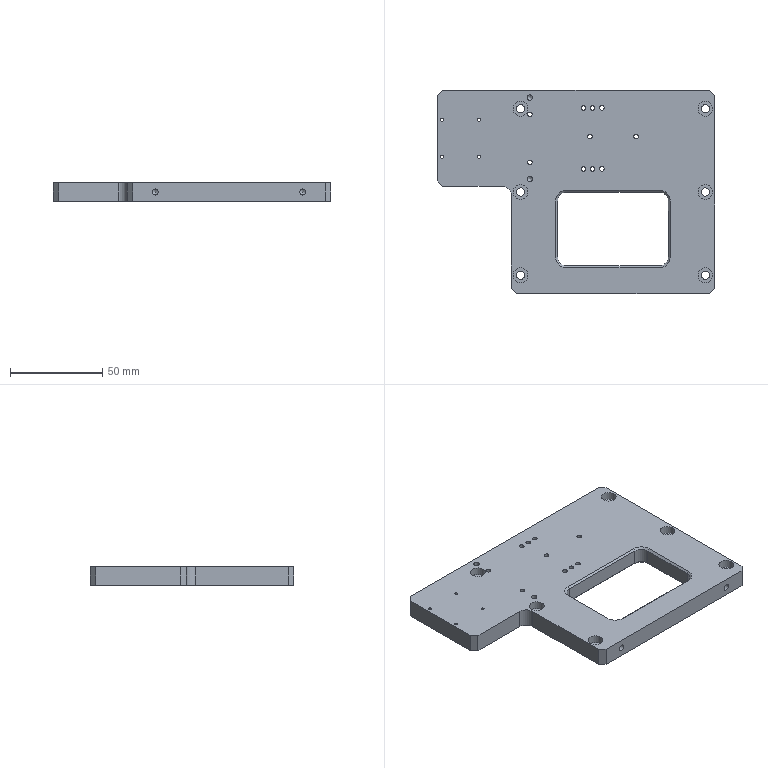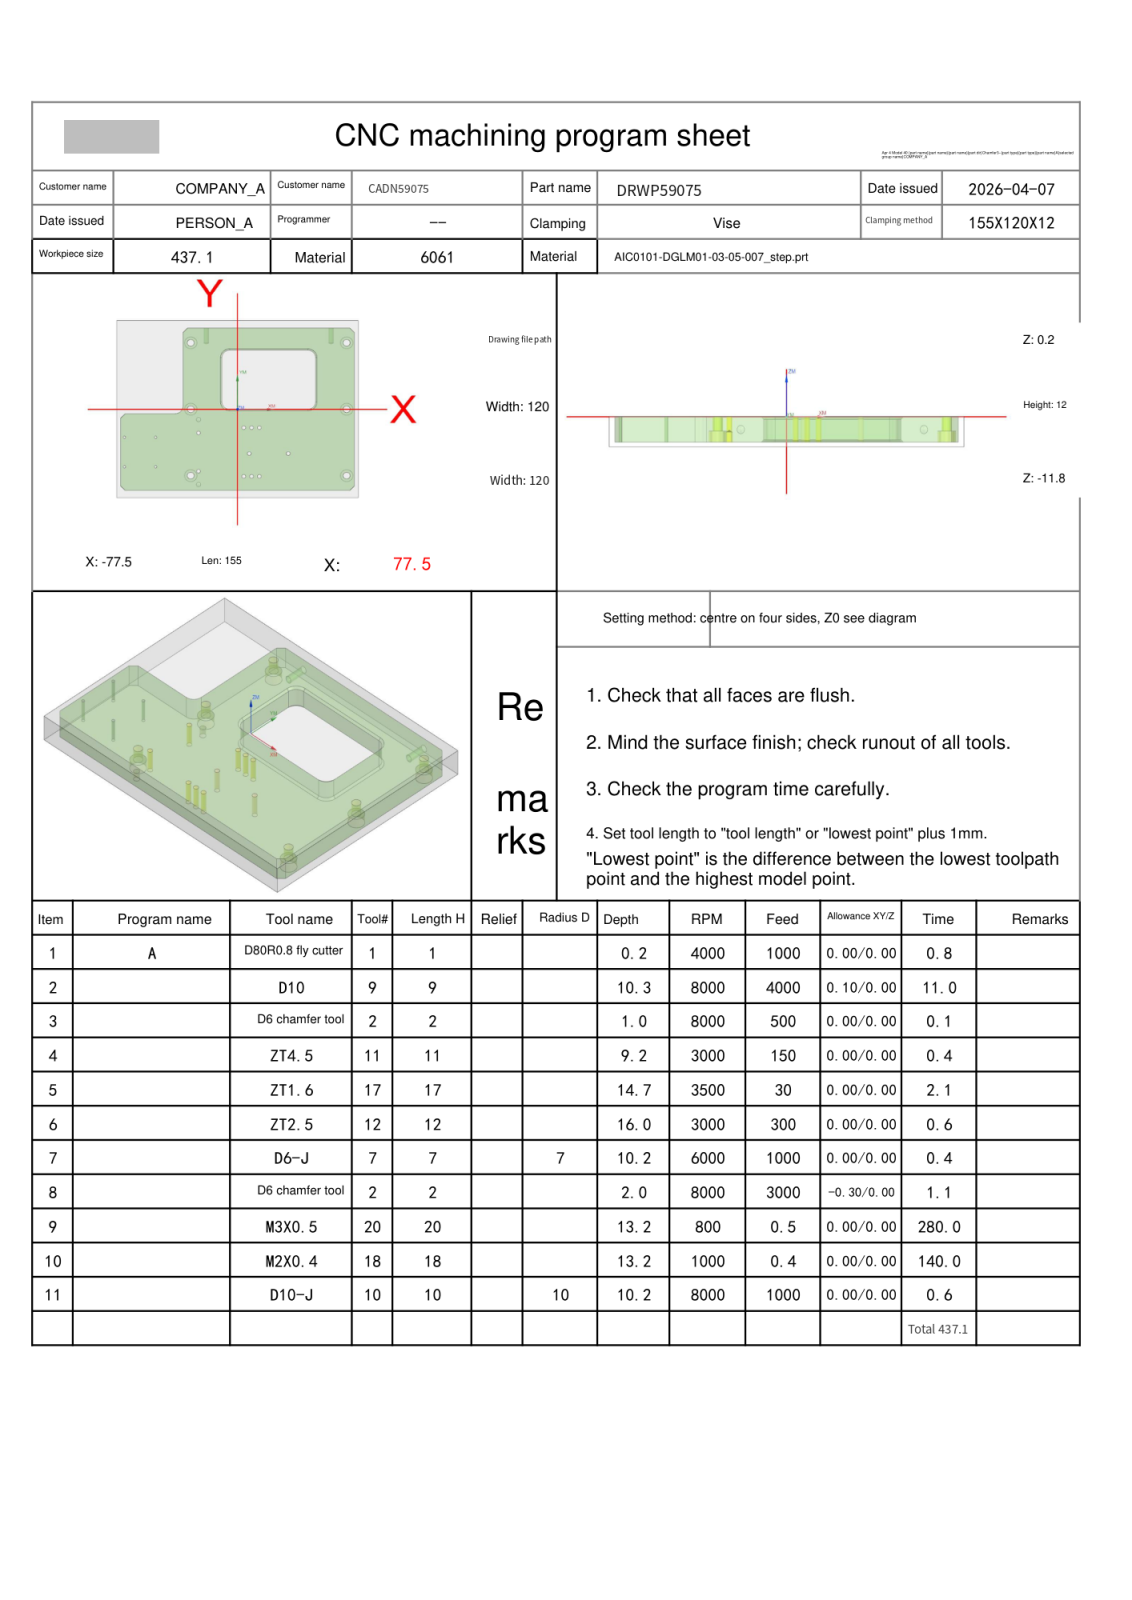NC program | NX | posted by the shop | part box 150 x 110 x 10 mm
Lines 1 to 40 of 3675:
%
O0001
(Machine time: 829.31 MIN)
(===Total Tool:10===)
(T1=D80R0.8 fly cutter D=80.  R=0.8  D-  H01 Z=0.    )
(T9=D10     D=10.  R=0.   D-  H09 Z=-10.1 )
(T2=D6 chamfer tool   D=6.   R=0.   D-  H02 Z=-1.75 )
(T11=ZT4.5  D=4.5  DR_a=118 D-  H11 Z=-8.95 )
(T17=ZT1.6  D=1.6  DR_a=118 D-  H17 Z=-14.48)
(T12=ZT2.5  D=2.5  DR_a=118 D-  H12 Z=-15.75)
(T7=D6-J    D=6.   R=0.   D7  H07 Z=-10.  )
(T20=M3X0.5 D=2.5  DR_a=180 D-  H20 Z=-13.  )
(T18=M2X0.4 D=1.6  DR_a=180 D-  H18 Z=-13.  )
(T10=D10-J  D=10.  R=0.   D10 H10 Z=-10.  )
G80 G90 G17 G49 G40
G91 G28 Z0
M01
N1 T01 M06
(D80R0.8 fly cutter  D=80. R=0.8 H=01 ce=0.00 di=0.00)
G00 G90 G54 X120. Y-47.5 M03 S4000
G43 H01 Z20.
M08
Z2.
G01 Z0.0 F1000.
X115.
X-115.
Y0.0
X115.
Y47.5
X-115.
X-120.
Z2.
G00 Z20.
G91 G28 Z0.0
M05
M09
G91 G28 Z0.0
M01